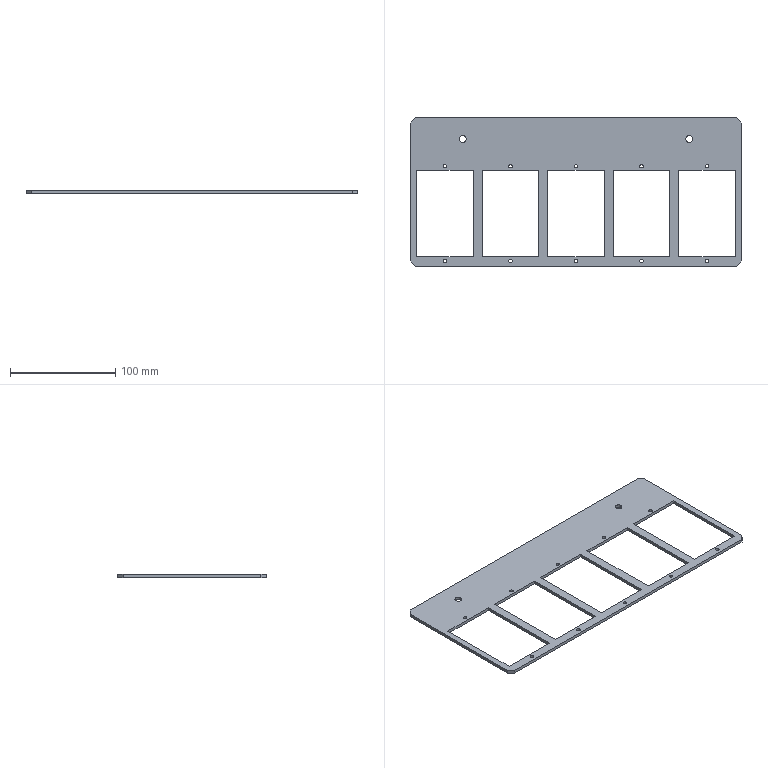Part | STEP file | 1 solid | 54 faces | box 315 x 141 x 3 mm | volume 66219 mm3 | plane 30 | cylinder 24 | commonest cylinder face diameters 3.3 x20 6.5 x4